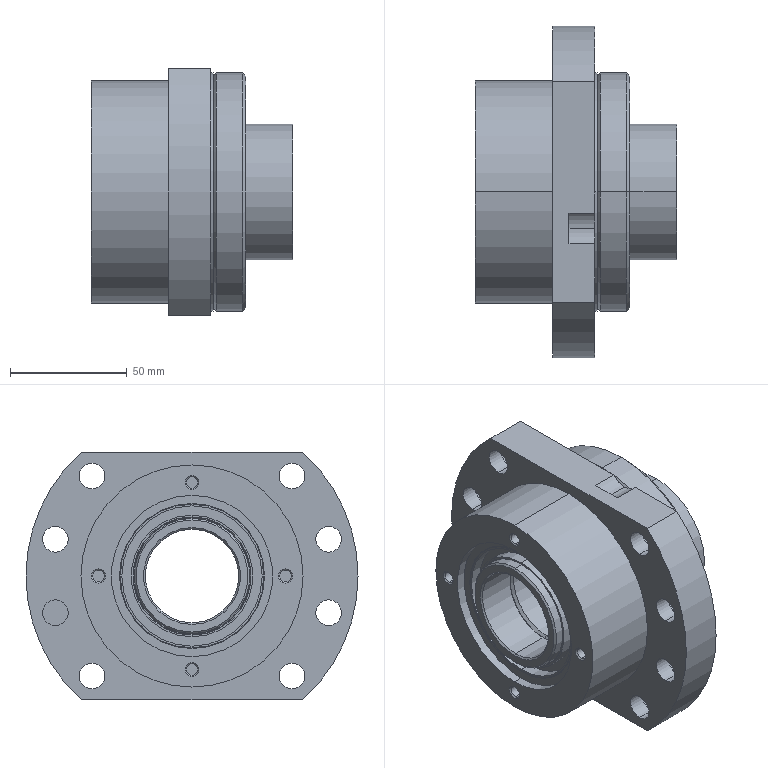Part | SolidWorks | features ICE 14, Revolution 8, RefAxis 5, CirPattern 4, LPattern 1, RevCut 1 | 1 solid | 317 faces | box 86 x 142 x 106 mm | volume 475751 mm3 | cylinder 130 | plane 113 | cone 74 | commonest cylinder face diameters 10 x16 10.98 x16 11 x16 17 x16 40 x10 4.917 x8